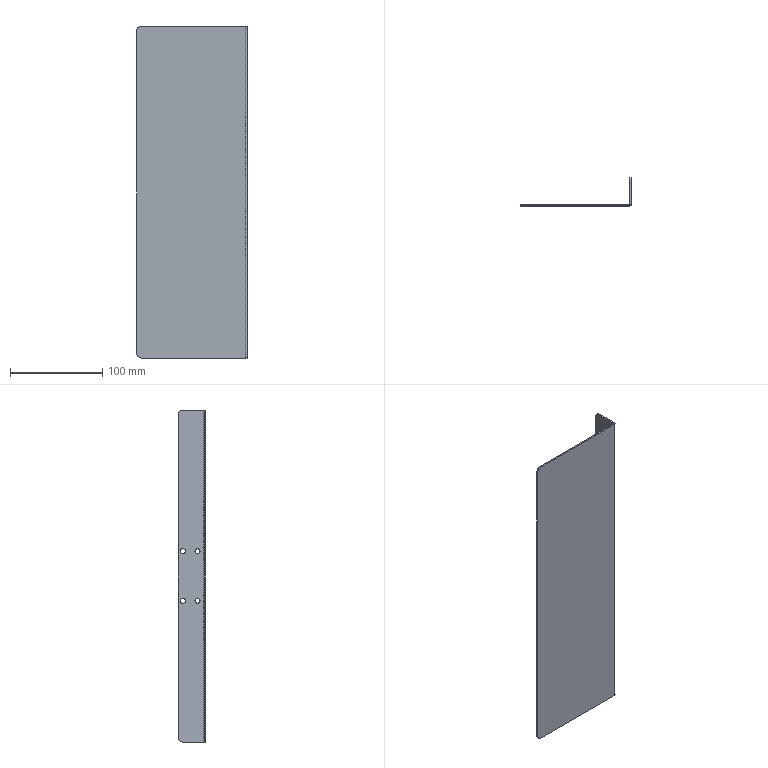Part | SolidWorks | features ExtruThin 1, Fillet 1, FlatPattern 1, FlattenBends 1, ICE 1, ProcessBends 1, SheetMetal 1 | 1 solid | 26 faces | box 120 x 30 x 360 mm | volume 79726 mm3 | cylinder 14 | plane 12 | commonest cylinder face diameters 5.5 x8 10 x4 1 x1 4 x1
STEP:
#1=CARTESIAN_POINT('',(0.,6.25,-27.));
#2=VERTEX_POINT('',#1);
#3=CARTESIAN_POINT('',(0.,11.75,-27.));
#4=VERTEX_POINT('',#3);
#5=CARTESIAN_POINT('',(0.,9.,-27.));
#6=DIRECTION('',(1.,0.,0.));
#7=DIRECTION('',(0.,1.,0.));
#8=AXIS2_PLACEMENT_3D('',#5,#6,#7);
#9=CIRCLE('',#8,2.75);
#10=EDGE_CURVE('',#2,#4,#9,.T.);
#11=ORIENTED_EDGE('',*,*,#10,.T.);
#12=CARTESIAN_POINT('',(-1.5,11.75,-27.));
#13=VERTEX_POINT('',#12);
#14=CARTESIAN_POINT('',(8.5,11.75,-27.));
#15=DIRECTION('',(-1.,0.,0.));
#16=VECTOR('',#15,1000.);
#17=LINE('',#14,#16);
#18=EDGE_CURVE('',#4,#13,#17,.T.);
#19=ORIENTED_EDGE('',*,*,#18,.T.);
#20=CARTESIAN_POINT('',(-1.5,6.25,-27.));
#21=VERTEX_POINT('',#20);
#22=CARTESIAN_POINT('',(-1.5,9.,-27.));
#23=DIRECTION('',(-1.,0.,0.));
#24=DIRECTION('',(0.,-1.,0.));
#25=AXIS2_PLACEMENT_3D('',#22,#23,#24);
#26=CIRCLE('',#25,2.75);
#27=EDGE_CURVE('',#13,#21,#26,.T.);
#28=ORIENTED_EDGE('',*,*,#27,.T.);
#29=CARTESIAN_POINT('',(8.5,6.25,-27.));
#30=DIRECTION('',(-1.,0.,0.));
#31=VECTOR('',#30,1000.);
#32=LINE('',#29,#31);
#33=EDGE_CURVE('',#2,#21,#32,.T.);
#34=ORIENTED_EDGE('',*,*,#33,.F.);
#35=EDGE_LOOP('',(#11,#19,#28,#34));
#36=FACE_OUTER_BOUND('',#35,.T.);
#37=CARTESIAN_POINT('',(8.5,9.,-27.));
#38=DIRECTION('',(-1.,0.,0.));
#39=DIRECTION('',(0.,-1.,0.));
#40=AXIS2_PLACEMENT_3D('',#37,#38,#39);
#41=CYLINDRICAL_SURFACE('',#40,2.75);
#42=ADVANCED_FACE('',(#36),#41,.F.);
#43=CARTESIAN_POINT('',(0.,6.25,27.));
#44=VERTEX_POINT('',#43);
#45=CARTESIAN_POINT('',(0.,11.75,27.));
#46=VERTEX_POINT('',#45);
#47=CARTESIAN_POINT('',(0.,9.,27.));
#48=DIRECTION('',(1.,0.,0.));
#49=DIRECTION('',(0.,1.,0.));
#50=AXIS2_PLACEMENT_3D('',#47,#48,#49);
#51=CIRCLE('',#50,2.75);
#52=EDGE_CURVE('',#44,#46,#51,.T.);
#53=ORIENTED_EDGE('',*,*,#52,.T.);
#54=CARTESIAN_POINT('',(-1.5,11.75,27.));
#55=VERTEX_POINT('',#54);
#56=CARTESIAN_POINT('',(8.5,11.75,27.));
#57=DIRECTION('',(-1.,0.,0.));
#58=VECTOR('',#57,1000.);
#59=LINE('',#56,#58);
#60=EDGE_CURVE('',#46,#55,#59,.T.);
#61=ORIENTED_EDGE('',*,*,#60,.T.);
#62=CARTESIAN_POINT('',(-1.5,6.25,27.));
#63=VERTEX_POINT('',#62);
#64=CARTESIAN_POINT('',(-1.5,9.,27.));
#65=DIRECTION('',(-1.,0.,0.));
#66=DIRECTION('',(0.,-1.,0.));
#67=AXIS2_PLACEMENT_3D('',#64,#65,#66);
#68=CIRCLE('',#67,2.75);
#69=EDGE_CURVE('',#55,#63,#68,.T.);
#70=ORIENTED_EDGE('',*,*,#69,.T.);
#71=CARTESIAN_POINT('',(8.5,6.25,27.));
#72=DIRECTION('',(-1.,0.,0.));
#73=VECTOR('',#72,1000.);
#74=LINE('',#71,#73);
#75=EDGE_CURVE('',#44,#63,#74,.T.);
#76=ORIENTED_EDGE('',*,*,#75,.F.);
#77=EDGE_LOOP('',(#53,#61,#70,#76));
#78=FACE_OUTER_BOUND('',#77,.T.);
#79=CARTESIAN_POINT('',(8.5,9.,27.));
#80=DIRECTION('',(-1.,0.,0.));
#81=DIRECTION('',(0.,-1.,0.));
#82=AXIS2_PLACEMENT_3D('',#79,#80,#81);
#83=CYLINDRICAL_SURFACE('',#82,2.75);
#84=ADVANCED_FACE('',(#78),#83,.F.);
#85=CARTESIAN_POINT('',(0.,22.25,27.));
#86=VERTEX_POINT('',#85);
#87=CARTESIAN_POINT('',(0.,27.75,27.));
#88=VERTEX_POINT('',#87);
#89=CARTESIAN_POINT('',(0.,25.,27.));
#90=DIRECTION('',(1.,0.,0.));
#91=DIRECTION('',(0.,1.,0.));
#92=AXIS2_PLACEMENT_3D('',#89,#90,#91);
#93=CIRCLE('',#92,2.75);
#94=EDGE_CURVE('',#86,#88,#93,.T.);
#95=ORIENTED_EDGE('',*,*,#94,.T.);
#96=CARTESIAN_POINT('',(-1.5,27.75,27.));
#97=VERTEX_POINT('',#96);
#98=CARTESIAN_POINT('',(8.5,27.75,27.));
#99=DIRECTION('',(-1.,0.,0.));
#100=VECTOR('',#99,1000.);
#101=LINE('',#98,#100);
#102=EDGE_CURVE('',#88,#97,#101,.T.);
#103=ORIENTED_EDGE('',*,*,#102,.T.);
#104=CARTESIAN_POINT('',(-1.5,22.25,27.));
#105=VERTEX_POINT('',#104);
#106=CARTESIAN_POINT('',(-1.5,25.,27.));
#107=DIRECTION('',(-1.,0.,0.));
#108=DIRECTION('',(0.,-1.,0.));
#109=AXIS2_PLACEMENT_3D('',#106,#107,#108);
#110=CIRCLE('',#109,2.75);
#111=EDGE_CURVE('',#97,#105,#110,.T.);
#112=ORIENTED_EDGE('',*,*,#111,.T.);
#113=CARTESIAN_POINT('',(8.5,22.25,27.));
#114=DIRECTION('',(-1.,0.,0.));
#115=VECTOR('',#114,1000.);
#116=LINE('',#113,#115);
#117=EDGE_CURVE('',#86,#105,#116,.T.);
#118=ORIENTED_EDGE('',*,*,#117,.F.);
#119=EDGE_LOOP('',(#95,#103,#112,#118));
#120=FACE_OUTER_BOUND('',#119,.T.);
#121=CARTESIAN_POINT('',(8.5,25.,27.));
#122=DIRECTION('',(-1.,0.,0.));
#123=DIRECTION('',(0.,-1.,0.));
#124=AXIS2_PLACEMENT_3D('',#121,#122,#123);
#125=CYLINDRICAL_SURFACE('',#124,2.75);
#126=ADVANCED_FACE('',(#120),#125,.F.);
#127=CARTESIAN_POINT('',(0.,22.25,-27.));
#128=VERTEX_POINT('',#127);
#129=CARTESIAN_POINT('',(0.,27.75,-27.));
#130=VERTEX_POINT('',#129);
#131=CARTESIAN_POINT('',(0.,25.,-27.));
#132=DIRECTION('',(1.,0.,0.));
#133=DIRECTION('',(0.,1.,0.));
#134=AXIS2_PLACEMENT_3D('',#131,#132,#133);
#135=CIRCLE('',#134,2.75);
#136=EDGE_CURVE('',#128,#130,#135,.T.);
#137=ORIENTED_EDGE('',*,*,#136,.T.);
#138=CARTESIAN_POINT('',(-1.5,27.75,-27.));
#139=VERTEX_POINT('',#138);
#140=CARTESIAN_POINT('',(8.5,27.75,-27.));
#141=DIRECTION('',(-1.,0.,0.));
#142=VECTOR('',#141,1000.);
#143=LINE('',#140,#142);
#144=EDGE_CURVE('',#130,#139,#143,.T.);
#145=ORIENTED_EDGE('',*,*,#144,.T.);
#146=CARTESIAN_POINT('',(-1.5,22.25,-27.));
#147=VERTEX_POINT('',#146);
#148=CARTESIAN_POINT('',(-1.5,25.,-27.));
#149=DIRECTION('',(-1.,0.,0.));
#150=DIRECTION('',(0.,-1.,0.));
#151=AXIS2_PLACEMENT_3D('',#148,#149,#150);
#152=CIRCLE('',#151,2.75);
#153=EDGE_CURVE('',#139,#147,#152,.T.);
#154=ORIENTED_EDGE('',*,*,#153,.T.);
#155=CARTESIAN_POINT('',(8.5,22.25,-27.));
#156=DIRECTION('',(-1.,0.,0.));
#157=VECTOR('',#156,1000.);
#158=LINE('',#155,#157);
#159=EDGE_CURVE('',#128,#147,#158,.T.);
#160=ORIENTED_EDGE('',*,*,#159,.F.);
#161=EDGE_LOOP('',(#137,#145,#154,#160));
#162=FACE_OUTER_BOUND('',#161,.T.);
#163=CARTESIAN_POINT('',(8.5,25.,-27.));
#164=DIRECTION('',(-1.,0.,0.));
#165=DIRECTION('',(0.,-1.,0.));
#166=AXIS2_PLACEMENT_3D('',#163,#164,#165);
#167=CYLINDRICAL_SURFACE('',#166,2.75);
#168=ADVANCED_FACE('',(#162),#167,.F.);
#169=ORIENTED_EDGE('',*,*,#144,.F.);
#170=CARTESIAN_POINT('',(0.,25.,-27.));
#171=DIRECTION('',(1.,0.,0.));
#172=DIRECTION('',(0.,1.,0.));
#173=AXIS2_PLACEMENT_3D('',#170,#171,#172);
#174=CIRCLE('',#173,2.75);
#175=EDGE_CURVE('',#130,#128,#174,.T.);
#176=ORIENTED_EDGE('',*,*,#175,.T.);
#177=ORIENTED_EDGE('',*,*,#159,.T.);
#178=CARTESIAN_POINT('',(-1.5,25.,-27.));
#179=DIRECTION('',(-1.,0.,0.));
#180=DIRECTION('',(0.,-1.,0.));
#181=AXIS2_PLACEMENT_3D('',#178,#179,#180);
#182=CIRCLE('',#181,2.75);
#183=EDGE_CURVE('',#147,#139,#182,.T.);
#184=ORIENTED_EDGE('',*,*,#183,.T.);
#185=EDGE_LOOP('',(#169,#176,#177,#184));
#186=FACE_OUTER_BOUND('',#185,.T.);
#187=CARTESIAN_POINT('',(8.5,25.,-27.));
#188=DIRECTION('',(-1.,0.,0.));
#189=DIRECTION('',(0.,-1.,0.));
#190=AXIS2_PLACEMENT_3D('',#187,#188,#189);
#191=CYLINDRICAL_SURFACE('',#190,2.75);
#192=ADVANCED_FACE('',(#186),#191,.F.);
#193=ORIENTED_EDGE('',*,*,#102,.F.);
#194=CARTESIAN_POINT('',(0.,25.,27.));
#195=DIRECTION('',(1.,0.,0.));
#196=DIRECTION('',(0.,1.,0.));
#197=AXIS2_PLACEMENT_3D('',#194,#195,#196);
#198=CIRCLE('',#197,2.75);
#199=EDGE_CURVE('',#88,#86,#198,.T.);
#200=ORIENTED_EDGE('',*,*,#199,.T.);
#201=ORIENTED_EDGE('',*,*,#117,.T.);
#202=CARTESIAN_POINT('',(-1.5,25.,27.));
#203=DIRECTION('',(-1.,0.,0.));
#204=DIRECTION('',(0.,-1.,0.));
#205=AXIS2_PLACEMENT_3D('',#202,#203,#204);
#206=CIRCLE('',#205,2.75);
#207=EDGE_CURVE('',#105,#97,#206,.T.);
#208=ORIENTED_EDGE('',*,*,#207,.T.);
#209=EDGE_LOOP('',(#193,#200,#201,#208));
#210=FACE_OUTER_BOUND('',#209,.T.);
#211=CARTESIAN_POINT('',(8.5,25.,27.));
#212=DIRECTION('',(-1.,0.,0.));
#213=DIRECTION('',(0.,-1.,0.));
#214=AXIS2_PLACEMENT_3D('',#211,#212,#213);
#215=CYLINDRICAL_SURFACE('',#214,2.75);
#216=ADVANCED_FACE('',(#210),#215,.F.);
#217=ORIENTED_EDGE('',*,*,#60,.F.);
#218=CARTESIAN_POINT('',(0.,9.,27.));
#219=DIRECTION('',(1.,0.,0.));
#220=DIRECTION('',(0.,1.,0.));
#221=AXIS2_PLACEMENT_3D('',#218,#219,#220);
#222=CIRCLE('',#221,2.75);
#223=EDGE_CURVE('',#46,#44,#222,.T.);
#224=ORIENTED_EDGE('',*,*,#223,.T.);
#225=ORIENTED_EDGE('',*,*,#75,.T.);
#226=CARTESIAN_POINT('',(-1.5,9.,27.));
#227=DIRECTION('',(-1.,0.,0.));
#228=DIRECTION('',(0.,-1.,0.));
#229=AXIS2_PLACEMENT_3D('',#226,#227,#228);
#230=CIRCLE('',#229,2.75);
#231=EDGE_CURVE('',#63,#55,#230,.T.);
#232=ORIENTED_EDGE('',*,*,#231,.T.);
#233=EDGE_LOOP('',(#217,#224,#225,#232));
#234=FACE_OUTER_BOUND('',#233,.T.);
#235=CARTESIAN_POINT('',(8.5,9.,27.));
#236=DIRECTION('',(-1.,0.,0.));
#237=DIRECTION('',(0.,-1.,0.));
#238=AXIS2_PLACEMENT_3D('',#235,#236,#237);
#239=CYLINDRICAL_SURFACE('',#238,2.75);
#240=ADVANCED_FACE('',(#234),#239,.F.);
#241=CARTESIAN_POINT('',(0.,2.,-180.));
#242=VERTEX_POINT('',#241);
#243=CARTESIAN_POINT('',(0.,2.,180.));
#244=VERTEX_POINT('',#243);
#245=CARTESIAN_POINT('',(0.,2.,180.));
#246=DIRECTION('',(0.,0.,1.));
#247=VECTOR('',#246,1000.);
#248=LINE('',#245,#247);
#249=EDGE_CURVE('',#242,#244,#248,.T.);
#250=ORIENTED_EDGE('',*,*,#249,.F.);
#251=CARTESIAN_POINT('',(0.,25.,-180.));
#252=VERTEX_POINT('',#251);
#253=CARTESIAN_POINT('',(0.,30.,-180.));
#254=DIRECTION('',(0.,-1.,0.));
#255=VECTOR('',#254,1000.);
#256=LINE('',#253,#255);
#257=EDGE_CURVE('',#252,#242,#256,.T.);
#258=ORIENTED_EDGE('',*,*,#257,.F.);
#259=CARTESIAN_POINT('',(0.,30.,-175.));
#260=VERTEX_POINT('',#259);
#261=CARTESIAN_POINT('',(0.,25.,-175.));
#262=DIRECTION('',(1.,0.,0.));
#263=DIRECTION('',(0.,1.,0.));
#264=AXIS2_PLACEMENT_3D('',#261,#262,#263);
#265=CIRCLE('',#264,5.);
#266=EDGE_CURVE('',#252,#260,#265,.T.);
#267=ORIENTED_EDGE('',*,*,#266,.T.);
#268=CARTESIAN_POINT('',(0.,30.,175.));
#269=VERTEX_POINT('',#268);
#270=CARTESIAN_POINT('',(0.,30.,180.));
#271=DIRECTION('',(0.,0.,-1.));
#272=VECTOR('',#271,1000.);
#273=LINE('',#270,#272);
#274=EDGE_CURVE('',#269,#260,#273,.T.);
#275=ORIENTED_EDGE('',*,*,#274,.F.);
#276=CARTESIAN_POINT('',(0.,25.,180.));
#277=VERTEX_POINT('',#276);
#278=CARTESIAN_POINT('',(0.,25.,175.));
#279=DIRECTION('',(1.,0.,0.));
#280=DIRECTION('',(0.,1.,0.));
#281=AXIS2_PLACEMENT_3D('',#278,#279,#280);
#282=CIRCLE('',#281,5.);
#283=EDGE_CURVE('',#269,#277,#282,.T.);
#284=ORIENTED_EDGE('',*,*,#283,.T.);
#285=CARTESIAN_POINT('',(0.,30.,180.));
#286=DIRECTION('',(0.,-1.,0.));
#287=VECTOR('',#286,1000.);
#288=LINE('',#285,#287);
#289=EDGE_CURVE('',#277,#244,#288,.T.);
#290=ORIENTED_EDGE('',*,*,#289,.T.);
#291=EDGE_LOOP('',(#250,#258,#267,#275,#284,#290));
#292=FACE_OUTER_BOUND('',#291,.T.);
#293=ORIENTED_EDGE('',*,*,#10,.F.);
#294=CARTESIAN_POINT('',(0.,9.,-27.));
#295=DIRECTION('',(1.,0.,0.));
#296=DIRECTION('',(0.,1.,0.));
#297=AXIS2_PLACEMENT_3D('',#294,#295,#296);
#298=CIRCLE('',#297,2.75);
#299=EDGE_CURVE('',#4,#2,#298,.T.);
#300=ORIENTED_EDGE('',*,*,#299,.F.);
#301=EDGE_LOOP('',(#293,#300));
#302=FACE_BOUND('',#301,.T.);
#303=ORIENTED_EDGE('',*,*,#52,.F.);
#304=ORIENTED_EDGE('',*,*,#223,.F.);
#305=EDGE_LOOP('',(#303,#304));
#306=FACE_BOUND('',#305,.T.);
#307=ORIENTED_EDGE('',*,*,#94,.F.);
#308=ORIENTED_EDGE('',*,*,#199,.F.);
#309=EDGE_LOOP('',(#307,#308));
#310=FACE_BOUND('',#309,.T.);
#311=ORIENTED_EDGE('',*,*,#136,.F.);
#312=ORIENTED_EDGE('',*,*,#175,.F.);
#313=EDGE_LOOP('',(#311,#312));
#314=FACE_BOUND('',#313,.T.);
#315=CARTESIAN_POINT('',(0.,30.,180.));
#316=DIRECTION('',(1.,0.,0.));
#317=DIRECTION('',(0.,1.,0.));
#318=AXIS2_PLACEMENT_3D('',#315,#316,#317);
#319=PLANE('',#318);
#320=ADVANCED_FACE('',(#292,#302,#306,#310,#314),#319,.T.);
#321=ORIENTED_EDGE('',*,*,#18,.F.);
#322=ORIENTED_EDGE('',*,*,#299,.T.);
#323=ORIENTED_EDGE('',*,*,#33,.T.);
#324=CARTESIAN_POINT('',(-1.5,9.,-27.));
#325=DIRECTION('',(-1.,0.,0.));
#326=DIRECTION('',(0.,-1.,0.));
#327=AXIS2_PLACEMENT_3D('',#324,#325,#326);
#328=CIRCLE('',#327,2.75);
#329=EDGE_CURVE('',#21,#13,#328,.T.);
#330=ORIENTED_EDGE('',*,*,#329,.T.);
#331=EDGE_LOOP('',(#321,#322,#323,#330));
#332=FACE_OUTER_BOUND('',#331,.T.);
#333=CARTESIAN_POINT('',(8.5,9.,-27.));
#334=DIRECTION('',(-1.,0.,0.));
#335=DIRECTION('',(0.,-1.,0.));
#336=AXIS2_PLACEMENT_3D('',#333,#334,#335);
#337=CYLINDRICAL_SURFACE('',#336,2.75);
#338=ADVANCED_FACE('',(#332),#337,.F.);
#339=ORIENTED_EDGE('',*,*,#329,.F.);
#340=ORIENTED_EDGE('',*,*,#27,.F.);
#341=EDGE_LOOP('',(#339,#340));
#342=FACE_BOUND('',#341,.T.);
#343=ORIENTED_EDGE('',*,*,#231,.F.);
#344=ORIENTED_EDGE('',*,*,#69,.F.);
#345=EDGE_LOOP('',(#343,#344));
#346=FACE_BOUND('',#345,.T.);
#347=ORIENTED_EDGE('',*,*,#207,.F.);
#348=ORIENTED_EDGE('',*,*,#111,.F.);
#349=EDGE_LOOP('',(#347,#348));
#350=FACE_BOUND('',#349,.T.);
#351=ORIENTED_EDGE('',*,*,#183,.F.);
#352=ORIENTED_EDGE('',*,*,#153,.F.);
#353=EDGE_LOOP('',(#351,#352));
#354=FACE_BOUND('',#353,.T.);
#355=CARTESIAN_POINT('',(-1.5,25.,-180.));
#356=VERTEX_POINT('',#355);
#357=CARTESIAN_POINT('',(-1.5,2.,-180.));
#358=VERTEX_POINT('',#357);
#359=CARTESIAN_POINT('',(-1.5,30.,-180.));
#360=DIRECTION('',(0.,-1.,0.));
#361=VECTOR('',#360,1000.);
#362=LINE('',#359,#361);
#363=EDGE_CURVE('',#356,#358,#362,.T.);
#364=ORIENTED_EDGE('',*,*,#363,.T.);
#365=CARTESIAN_POINT('',(-1.5,2.,180.));
#366=VERTEX_POINT('',#365);
#367=CARTESIAN_POINT('',(-1.5,2.,180.));
#368=DIRECTION('',(0.,0.,1.));
#369=VECTOR('',#368,1000.);
#370=LINE('',#367,#369);
#371=EDGE_CURVE('',#358,#366,#370,.T.);
#372=ORIENTED_EDGE('',*,*,#371,.T.);
#373=CARTESIAN_POINT('',(-1.5,25.,180.));
#374=VERTEX_POINT('',#373);
#375=CARTESIAN_POINT('',(-1.5,30.,180.));
#376=DIRECTION('',(0.,-1.,0.));
#377=VECTOR('',#376,1000.);
#378=LINE('',#375,#377);
#379=EDGE_CURVE('',#374,#366,#378,.T.);
#380=ORIENTED_EDGE('',*,*,#379,.F.);
#381=CARTESIAN_POINT('',(-1.5,30.,175.));
#382=VERTEX_POINT('',#381);
#383=CARTESIAN_POINT('',(-1.5,25.,175.));
#384=DIRECTION('',(-1.,0.,0.));
#385=DIRECTION('',(0.,1.,0.));
#386=AXIS2_PLACEMENT_3D('',#383,#384,#385);
#387=CIRCLE('',#386,5.);
#388=EDGE_CURVE('',#374,#382,#387,.T.);
#389=ORIENTED_EDGE('',*,*,#388,.T.);
#390=CARTESIAN_POINT('',(-1.5,30.,-175.));
#391=VERTEX_POINT('',#390);
#392=CARTESIAN_POINT('',(-1.5,30.,180.));
#393=DIRECTION('',(0.,0.,-1.));
#394=VECTOR('',#393,1000.);
#395=LINE('',#392,#394);
#396=EDGE_CURVE('',#382,#391,#395,.T.);
#397=ORIENTED_EDGE('',*,*,#396,.T.);
#398=CARTESIAN_POINT('',(-1.5,25.,-175.));
#399=DIRECTION('',(-1.,0.,0.));
#400=DIRECTION('',(0.,1.,0.));
#401=AXIS2_PLACEMENT_3D('',#398,#399,#400);
#402=CIRCLE('',#401,5.);
#403=EDGE_CURVE('',#391,#356,#402,.T.);
#404=ORIENTED_EDGE('',*,*,#403,.T.);
#405=EDGE_LOOP('',(#364,#372,#380,#389,#397,#404));
#406=FACE_OUTER_BOUND('',#405,.T.);
#407=CARTESIAN_POINT('',(-1.5,30.,180.));
#408=DIRECTION('',(1.,0.,0.));
#409=DIRECTION('',(0.,1.,0.));
#410=AXIS2_PLACEMENT_3D('',#407,#408,#409);
#411=PLANE('',#410);
#412=ADVANCED_FACE('',(#342,#346,#350,#354,#406),#411,.F.);
#413=CARTESIAN_POINT('',(-723.674,2.,180.));
#414=DIRECTION('',(1.,0.,0.));
#415=VECTOR('',#414,1000.);
#416=LINE('',#413,#415);
#417=EDGE_CURVE('',#366,#244,#416,.T.);
#418=ORIENTED_EDGE('',*,*,#417,.T.);
#419=ORIENTED_EDGE('',*,*,#289,.F.);
#420=CARTESIAN_POINT('',(-723.674,25.,180.));
#421=DIRECTION('',(1.,0.,0.));
#422=VECTOR('',#421,1000.);
#423=LINE('',#420,#422);
#424=EDGE_CURVE('',#374,#277,#423,.T.);
#425=ORIENTED_EDGE('',*,*,#424,.F.);
#426=ORIENTED_EDGE('',*,*,#379,.T.);
#427=EDGE_LOOP('',(#418,#419,#425,#426));
#428=FACE_OUTER_BOUND('',#427,.T.);
#429=CARTESIAN_POINT('',(-723.674,30.,180.));
#430=DIRECTION('',(0.,0.,1.));
#431=DIRECTION('',(0.,1.,0.));
#432=AXIS2_PLACEMENT_3D('',#429,#430,#431);
#433=PLANE('',#432);
#434=ADVANCED_FACE('',(#428),#433,.T.);
#435=ORIENTED_EDGE('',*,*,#283,.F.);
#436=CARTESIAN_POINT('',(-723.674,30.,175.));
#437=DIRECTION('',(1.,0.,0.));
#438=VECTOR('',#437,1000.);
#439=LINE('',#436,#438);
#440=EDGE_CURVE('',#382,#269,#439,.T.);
#441=ORIENTED_EDGE('',*,*,#440,.F.);
#442=ORIENTED_EDGE('',*,*,#388,.F.);
#443=ORIENTED_EDGE('',*,*,#424,.T.);
#444=EDGE_LOOP('',(#435,#441,#442,#443));
#445=FACE_OUTER_BOUND('',#444,.T.);
#446=CARTESIAN_POINT('',(-723.674,25.,175.));
#447=DIRECTION('',(1.,0.,0.));
#448=DIRECTION('',(0.,1.,0.));
#449=AXIS2_PLACEMENT_3D('',#446,#447,#448);
#450=CYLINDRICAL_SURFACE('',#449,5.);
#451=ADVANCED_FACE('',(#445),#450,.T.);
#452=ORIENTED_EDGE('',*,*,#274,.T.);
#453=CARTESIAN_POINT('',(-723.674,30.,-175.));
#454=DIRECTION('',(1.,0.,0.));
#455=VECTOR('',#454,1000.);
#456=LINE('',#453,#455);
#457=EDGE_CURVE('',#391,#260,#456,.T.);
#458=ORIENTED_EDGE('',*,*,#457,.F.);
#459=ORIENTED_EDGE('',*,*,#396,.F.);
#460=ORIENTED_EDGE('',*,*,#440,.T.);
#461=EDGE_LOOP('',(#452,#458,#459,#460));
#462=FACE_OUTER_BOUND('',#461,.T.);
#463=CARTESIAN_POINT('',(-723.674,30.,180.));
#464=DIRECTION('',(0.,-1.,0.));
#465=DIRECTION('',(1.,0.,0.));
#466=AXIS2_PLACEMENT_3D('',#463,#464,#465);
#467=PLANE('',#466);
#468=ADVANCED_FACE('',(#462),#467,.F.);
#469=ORIENTED_EDGE('',*,*,#266,.F.);
#470=CARTESIAN_POINT('',(-723.674,25.,-180.));
#471=DIRECTION('',(1.,0.,0.));
#472=VECTOR('',#471,1000.);
#473=LINE('',#470,#472);
#474=EDGE_CURVE('',#356,#252,#473,.T.);
#475=ORIENTED_EDGE('',*,*,#474,.F.);
#476=ORIENTED_EDGE('',*,*,#403,.F.);
#477=ORIENTED_EDGE('',*,*,#457,.T.);
#478=EDGE_LOOP('',(#469,#475,#476,#477));
#479=FACE_OUTER_BOUND('',#478,.T.);
#480=CARTESIAN_POINT('',(-723.674,25.,-175.));
#481=DIRECTION('',(1.,0.,0.));
#482=DIRECTION('',(0.,1.,0.));
#483=AXIS2_PLACEMENT_3D('',#480,#481,#482);
#484=CYLINDRICAL_SURFACE('',#483,5.);
#485=ADVANCED_FACE('',(#479),#484,.T.);
#486=ORIENTED_EDGE('',*,*,#257,.T.);
#487=CARTESIAN_POINT('',(-723.674,2.,-180.));
#488=DIRECTION('',(1.,0.,0.));
#489=VECTOR('',#488,1000.);
#490=LINE('',#487,#489);
#491=EDGE_CURVE('',#358,#242,#490,.T.);
#492=ORIENTED_EDGE('',*,*,#491,.F.);
#493=ORIENTED_EDGE('',*,*,#363,.F.);
#494=ORIENTED_EDGE('',*,*,#474,.T.);
#495=EDGE_LOOP('',(#486,#492,#493,#494));
#496=FACE_OUTER_BOUND('',#495,.T.);
#497=CARTESIAN_POINT('',(-723.674,30.,-180.));
#498=DIRECTION('',(0.,0.,1.));
#499=DIRECTION('',(0.,1.,0.));
#500=AXIS2_PLACEMENT_3D('',#497,#498,#499);
#501=PLANE('',#500);
#502=ADVANCED_FACE('',(#496),#501,.F.);
#503=CARTESIAN_POINT('',(-115.,0.,180.));
#504=VERTEX_POINT('',#503);
#505=CARTESIAN_POINT('',(-120.,0.,175.));
#506=VERTEX_POINT('',#505);
#507=CARTESIAN_POINT('',(-115.,0.,175.));
#508=DIRECTION('',(0.,-1.,0.));
#509=DIRECTION('',(1.,0.,0.));
#510=AXIS2_PLACEMENT_3D('',#507,#508,#509);
#511=CIRCLE('',#510,5.);
#512=EDGE_CURVE('',#504,#506,#511,.T.);
#513=ORIENTED_EDGE('',*,*,#512,.F.);
#514=CARTESIAN_POINT('',(-115.,1.5,180.));
#515=VERTEX_POINT('',#514);
#516=CARTESIAN_POINT('',(-115.,759.191,180.));
#517=DIRECTION('',(0.,-1.,0.));
#518=VECTOR('',#517,1000.);
#519=LINE('',#516,#518);
#520=EDGE_CURVE('',#515,#504,#519,.T.);
#521=ORIENTED_EDGE('',*,*,#520,.F.);
#522=CARTESIAN_POINT('',(-120.,1.5,175.));
#523=VERTEX_POINT('',#522);
#524=CARTESIAN_POINT('',(-115.,1.5,175.));
#525=DIRECTION('',(0.,1.,0.));
#526=DIRECTION('',(1.,0.,0.));
#527=AXIS2_PLACEMENT_3D('',#524,#525,#526);
#528=CIRCLE('',#527,5.);
#529=EDGE_CURVE('',#523,#515,#528,.T.);
#530=ORIENTED_EDGE('',*,*,#529,.F.);
#531=CARTESIAN_POINT('',(-120.,759.191,175.));
#532=DIRECTION('',(0.,-1.,0.));
#533=VECTOR('',#532,1000.);
#534=LINE('',#531,#533);
#535=EDGE_CURVE('',#523,#506,#534,.T.);
#536=ORIENTED_EDGE('',*,*,#535,.T.);
#537=EDGE_LOOP('',(#513,#521,#530,#536));
#538=FACE_OUTER_BOUND('',#537,.T.);
#539=CARTESIAN_POINT('',(-115.,759.191,175.));
#540=DIRECTION('',(0.,-1.,0.));
#541=DIRECTION('',(1.,0.,0.));
#542=AXIS2_PLACEMENT_3D('',#539,#540,#541);
#543=CYLINDRICAL_SURFACE('',#542,5.);
#544=ADVANCED_FACE('',(#538),#543,.T.);
#545=CARTESIAN_POINT('',(-120.,1.5,-175.));
#546=VERTEX_POINT('',#545);
#547=CARTESIAN_POINT('',(-120.,0.,-175.));
#548=VERTEX_POINT('',#547);
#549=CARTESIAN_POINT('',(-120.,759.191,-175.));
#550=DIRECTION('',(0.,-1.,0.));
#551=VECTOR('',#550,1000.);
#552=LINE('',#549,#551);
#553=EDGE_CURVE('',#546,#548,#552,.T.);
#554=ORIENTED_EDGE('',*,*,#553,.T.);
#555=CARTESIAN_POINT('',(-120.,0.,180.));
#556=DIRECTION('',(0.,0.,-1.));
#557=VECTOR('',#556,1000.);
#558=LINE('',#555,#557);
#559=EDGE_CURVE('',#506,#548,#558,.T.);
#560=ORIENTED_EDGE('',*,*,#559,.F.);
#561=ORIENTED_EDGE('',*,*,#535,.F.);
#562=CARTESIAN_POINT('',(-120.,1.5,180.));
#563=DIRECTION('',(0.,0.,-1.));
#564=VECTOR('',#563,1000.);
#565=LINE('',#562,#564);
#566=EDGE_CURVE('',#523,#546,#565,.T.);
#567=ORIENTED_EDGE('',*,*,#566,.T.);
#568=EDGE_LOOP('',(#554,#560,#561,#567));
#569=FACE_OUTER_BOUND('',#568,.T.);
#570=CARTESIAN_POINT('',(-120.,759.191,180.));
#571=DIRECTION('',(-1.,0.,0.));
#572=DIRECTION('',(0.,-1.,0.));
#573=AXIS2_PLACEMENT_3D('',#570,#571,#572);
#574=PLANE('',#573);
#575=ADVANCED_FACE('',(#569),#574,.T.);
#576=CARTESIAN_POINT('',(-115.,0.,-180.));
#577=VERTEX_POINT('',#576);
#578=CARTESIAN_POINT('',(-115.,0.,-175.));
#579=DIRECTION('',(0.,-1.,0.));
#580=DIRECTION('',(1.,0.,0.));
#581=AXIS2_PLACEMENT_3D('',#578,#579,#580);
#582=CIRCLE('',#581,5.);
#583=EDGE_CURVE('',#548,#577,#582,.T.);
#584=ORIENTED_EDGE('',*,*,#583,.F.);
#585=ORIENTED_EDGE('',*,*,#553,.F.);
#586=CARTESIAN_POINT('',(-115.,1.5,-180.));
#587=VERTEX_POINT('',#586);
#588=CARTESIAN_POINT('',(-115.,1.5,-175.));
#589=DIRECTION('',(0.,1.,0.));
#590=DIRECTION('',(1.,0.,0.));
#591=AXIS2_PLACEMENT_3D('',#588,#589,#590);
#592=CIRCLE('',#591,5.);
#593=EDGE_CURVE('',#587,#546,#592,.T.);
#594=ORIENTED_EDGE('',*,*,#593,.F.);
#595=CARTESIAN_POINT('',(-115.,759.191,-180.));
#596=DIRECTION('',(0.,-1.,0.));
#597=VECTOR('',#596,1000.);
#598=LINE('',#595,#597);
#599=EDGE_CURVE('',#587,#577,#598,.T.);
#600=ORIENTED_EDGE('',*,*,#599,.T.);
#601=EDGE_LOOP('',(#584,#585,#594,#600));
#602=FACE_OUTER_BOUND('',#601,.T.);
#603=CARTESIAN_POINT('',(-115.,759.191,-175.));
#604=DIRECTION('',(0.,-1.,0.));
#605=DIRECTION('',(1.,0.,0.));
#606=AXIS2_PLACEMENT_3D('',#603,#604,#605);
#607=CYLINDRICAL_SURFACE('',#606,5.);
#608=ADVANCED_FACE('',(#602),#607,.T.);
#609=CARTESIAN_POINT('',(-2.,1.5,-180.));
#610=VERTEX_POINT('',#609);
#611=CARTESIAN_POINT('',(-2.,1.5,180.));
#612=VERTEX_POINT('',#611);
#613=CARTESIAN_POINT('',(-2.,1.5,180.));
#614=DIRECTION('',(0.,0.,1.));
#615=VECTOR('',#614,1000.);
#616=LINE('',#613,#615);
#617=EDGE_CURVE('',#610,#612,#616,.T.);
#618=ORIENTED_EDGE('',*,*,#617,.F.);
#619=CARTESIAN_POINT('',(0.,1.5,-180.));
#620=DIRECTION('',(-1.,0.,0.));
#621=VECTOR('',#620,1000.);
#622=LINE('',#619,#621);
#623=EDGE_CURVE('',#610,#587,#622,.T.);
#624=ORIENTED_EDGE('',*,*,#623,.T.);
#625=ORIENTED_EDGE('',*,*,#593,.T.);
#626=ORIENTED_EDGE('',*,*,#566,.F.);
#627=ORIENTED_EDGE('',*,*,#529,.T.);
#628=CARTESIAN_POINT('',(0.,1.5,180.));
#629=DIRECTION('',(-1.,0.,0.));
#630=VECTOR('',#629,1000.);
#631=LINE('',#628,#630);
#632=EDGE_CURVE('',#612,#515,#631,.T.);
#633=ORIENTED_EDGE('',*,*,#632,.F.);
#634=EDGE_LOOP('',(#618,#624,#625,#626,#627,#633));
#635=FACE_OUTER_BOUND('',#634,.T.);
#636=CARTESIAN_POINT('',(0.,1.5,180.));
#637=DIRECTION('',(0.,-1.,0.));
#638=DIRECTION('',(1.,0.,0.));
#639=AXIS2_PLACEMENT_3D('',#636,#637,#638);
#640=PLANE('',#639);
#641=ADVANCED_FACE('',(#635),#640,.F.);
#642=CARTESIAN_POINT('',(-2.,0.,-180.));
#643=VERTEX_POINT('',#642);
#644=CARTESIAN_POINT('',(0.,0.,-180.));
#645=DIRECTION('',(-1.,0.,0.));
#646=VECTOR('',#645,1000.);
#647=LINE('',#644,#646);
#648=EDGE_CURVE('',#643,#577,#647,.T.);
#649=ORIENTED_EDGE('',*,*,#648,.T.);
#650=ORIENTED_EDGE('',*,*,#599,.F.);
#651=ORIENTED_EDGE('',*,*,#623,.F.);
#652=CARTESIAN_POINT('',(-2.,759.191,-180.));
#653=DIRECTION('',(0.,-1.,0.));
#654=VECTOR('',#653,1000.);
#655=LINE('',#652,#654);
#656=EDGE_CURVE('',#610,#643,#655,.T.);
#657=ORIENTED_EDGE('',*,*,#656,.T.);
#658=EDGE_LOOP('',(#649,#650,#651,#657));
#659=FACE_OUTER_BOUND('',#658,.T.);
#660=CARTESIAN_POINT('',(0.,759.191,-180.));
#661=DIRECTION('',(0.,0.,1.));
#662=DIRECTION('',(1.,0.,0.));
#663=AXIS2_PLACEMENT_3D('',#660,#661,#662);
#664=PLANE('',#663);
#665=ADVANCED_FACE('',(#659),#664,.F.);
#666=ORIENTED_EDGE('',*,*,#648,.F.);
#667=CARTESIAN_POINT('',(-2.,0.,180.));
#668=VERTEX_POINT('',#667);
#669=CARTESIAN_POINT('',(-2.,0.,180.));
#670=DIRECTION('',(0.,0.,1.));
#671=VECTOR('',#670,1000.);
#672=LINE('',#669,#671);
#673=EDGE_CURVE('',#643,#668,#672,.T.);
#674=ORIENTED_EDGE('',*,*,#673,.T.);
#675=CARTESIAN_POINT('',(0.,0.,180.));
#676=DIRECTION('',(-1.,0.,0.));
#677=VECTOR('',#676,1000.);
#678=LINE('',#675,#677);
#679=EDGE_CURVE('',#668,#504,#678,.T.);
#680=ORIENTED_EDGE('',*,*,#679,.T.);
#681=ORIENTED_EDGE('',*,*,#512,.T.);
#682=ORIENTED_EDGE('',*,*,#559,.T.);
#683=ORIENTED_EDGE('',*,*,#583,.T.);
#684=EDGE_LOOP('',(#666,#674,#680,#681,#682,#683));
#685=FACE_OUTER_BOUND('',#684,.T.);
#686=CARTESIAN_POINT('',(0.,0.,180.));
#687=DIRECTION('',(0.,-1.,0.));
#688=DIRECTION('',(1.,0.,0.));
#689=AXIS2_PLACEMENT_3D('',#686,#687,#688);
#690=PLANE('',#689);
#691=ADVANCED_FACE('',(#685),#690,.T.);
#692=ORIENTED_EDGE('',*,*,#520,.T.);
#693=ORIENTED_EDGE('',*,*,#679,.F.);
#694=CARTESIAN_POINT('',(-2.,759.191,180.));
#695=DIRECTION('',(0.,-1.,0.));
#696=VECTOR('',#695,1000.);
#697=LINE('',#694,#696);
#698=EDGE_CURVE('',#612,#668,#697,.T.);
#699=ORIENTED_EDGE('',*,*,#698,.F.);
#700=ORIENTED_EDGE('',*,*,#632,.T.);
#701=EDGE_LOOP('',(#692,#693,#699,#700));
#702=FACE_OUTER_BOUND('',#701,.T.);
#703=CARTESIAN_POINT('',(0.,759.191,180.));
#704=DIRECTION('',(0.,0.,1.));
#705=DIRECTION('',(1.,0.,0.));
#706=AXIS2_PLACEMENT_3D('',#703,#704,#705);
#707=PLANE('',#706);
#708=ADVANCED_FACE('',(#702),#707,.T.);
#709=ORIENTED_EDGE('',*,*,#417,.F.);
#710=CARTESIAN_POINT('',(-2.,2.,180.));
#711=DIRECTION('',(0.,0.,-1.));
#712=DIRECTION('',(-1.,0.,0.));
#713=AXIS2_PLACEMENT_3D('',#710,#711,#712);
#714=CIRCLE('',#713,0.5);
#715=EDGE_CURVE('',#366,#612,#714,.T.);
#716=ORIENTED_EDGE('',*,*,#715,.T.);
#717=ORIENTED_EDGE('',*,*,#698,.T.);
#718=CARTESIAN_POINT('',(-2.,2.,180.));
#719=DIRECTION('',(0.,0.,-1.));
#720=DIRECTION('',(-1.,0.,0.));
#721=AXIS2_PLACEMENT_3D('',#718,#719,#720);
#722=CIRCLE('',#721,2.);
#723=EDGE_CURVE('',#244,#668,#722,.T.);
#724=ORIENTED_EDGE('',*,*,#723,.F.);
#725=EDGE_LOOP('',(#709,#716,#717,#724));
#726=FACE_OUTER_BOUND('',#725,.T.);
#727=CARTESIAN_POINT('',(-2.,2.,180.));
#728=DIRECTION('',(0.,0.,1.));
#729=DIRECTION('',(1.,0.,0.));
#730=AXIS2_PLACEMENT_3D('',#727,#728,#729);
#731=PLANE('',#730);
#732=ADVANCED_FACE('',(#726),#731,.T.);
#733=CARTESIAN_POINT('',(-2.,2.,-180.));
#734=DIRECTION('',(0.,0.,1.));
#735=DIRECTION('',(-1.,0.,0.));
#736=AXIS2_PLACEMENT_3D('',#733,#734,#735);
#737=CIRCLE('',#736,0.5);
#738=EDGE_CURVE('',#610,#358,#737,.T.);
#739=ORIENTED_EDGE('',*,*,#738,.T.);
#740=ORIENTED_EDGE('',*,*,#491,.T.);
#741=CARTESIAN_POINT('',(-2.,2.,-180.));
#742=DIRECTION('',(0.,0.,1.));
#743=DIRECTION('',(-1.,0.,0.));
#744=AXIS2_PLACEMENT_3D('',#741,#742,#743);
#745=CIRCLE('',#744,2.);
#746=EDGE_CURVE('',#643,#242,#745,.T.);
#747=ORIENTED_EDGE('',*,*,#746,.F.);
#748=ORIENTED_EDGE('',*,*,#656,.F.);
#749=EDGE_LOOP('',(#739,#740,#747,#748));
#750=FACE_OUTER_BOUND('',#749,.T.);
#751=CARTESIAN_POINT('',(-2.,2.,-180.));
#752=DIRECTION('',(0.,0.,-1.));
#753=DIRECTION('',(-1.,0.,0.));
#754=AXIS2_PLACEMENT_3D('',#751,#752,#753);
#755=PLANE('',#754);
#756=ADVANCED_FACE('',(#750),#755,.T.);
#757=ORIENTED_EDGE('',*,*,#673,.F.);
#758=ORIENTED_EDGE('',*,*,#746,.T.);
#759=ORIENTED_EDGE('',*,*,#249,.T.);
#760=ORIENTED_EDGE('',*,*,#723,.T.);
#761=EDGE_LOOP('',(#757,#758,#759,#760));
#762=FACE_OUTER_BOUND('',#761,.T.);
#763=CARTESIAN_POINT('',(-2.,2.,569.188));
#764=DIRECTION('',(0.,0.,-1.));
#765=DIRECTION('',(-1.,0.,0.));
#766=AXIS2_PLACEMENT_3D('',#763,#764,#765);
#767=CYLINDRICAL_SURFACE('',#766,2.);
#768=ADVANCED_FACE('',(#762),#767,.T.);
#769=ORIENTED_EDGE('',*,*,#617,.T.);
#770=ORIENTED_EDGE('',*,*,#715,.F.);
#771=ORIENTED_EDGE('',*,*,#371,.F.);
#772=ORIENTED_EDGE('',*,*,#738,.F.);
#773=EDGE_LOOP('',(#769,#770,#771,#772));
#774=FACE_OUTER_BOUND('',#773,.T.);
#775=CARTESIAN_POINT('',(-2.,2.,569.188));
#776=DIRECTION('',(0.,0.,-1.));
#777=DIRECTION('',(-1.,0.,0.));
#778=AXIS2_PLACEMENT_3D('',#775,#776,#777);
#779=CYLINDRICAL_SURFACE('',#778,0.5);
#780=ADVANCED_FACE('',(#774),#779,.F.);
#781=CLOSED_SHELL('',(#42,#84,#126,#168,#192,#216,#240,#320,#338,#412,#434,#451,#468,#485,#502,#544,#575,#608,#641,#665,#691,#708,#732,#756,#768,#780));
#782=MANIFOLD_SOLID_BREP('',#781);
#783=CARTESIAN_POINT('',(0.,0.,0.));
#784=DIRECTION('',(0.,0.,1.));
#785=DIRECTION('',(1.,0.,0.));
#786=AXIS2_PLACEMENT_3D('',#783,#784,#785);
#787=(LENGTH_UNIT()NAMED_UNIT(*)SI_UNIT(.MILLI.,.METRE.));
#788=UNCERTAINTY_MEASURE_WITH_UNIT(LENGTH_MEASURE(0.00001),#787,'','');
#789=(NAMED_UNIT(*)PLANE_ANGLE_UNIT()SI_UNIT($,.RADIAN.));
#790=(NAMED_UNIT(*)SI_UNIT($,.STERADIAN.)SOLID_ANGLE_UNIT());
#791=(GEOMETRIC_REPRESENTATION_CONTEXT(3)GLOBAL_UNCERTAINTY_ASSIGNED_CONTEXT((#788))GLOBAL_UNIT_ASSIGNED_CONTEXT((#787,#789,#790))REPRESENTATION_CONTEXT('',''));
#792=ADVANCED_BREP_SHAPE_REPRESENTATION('',(#782,#786),#791);